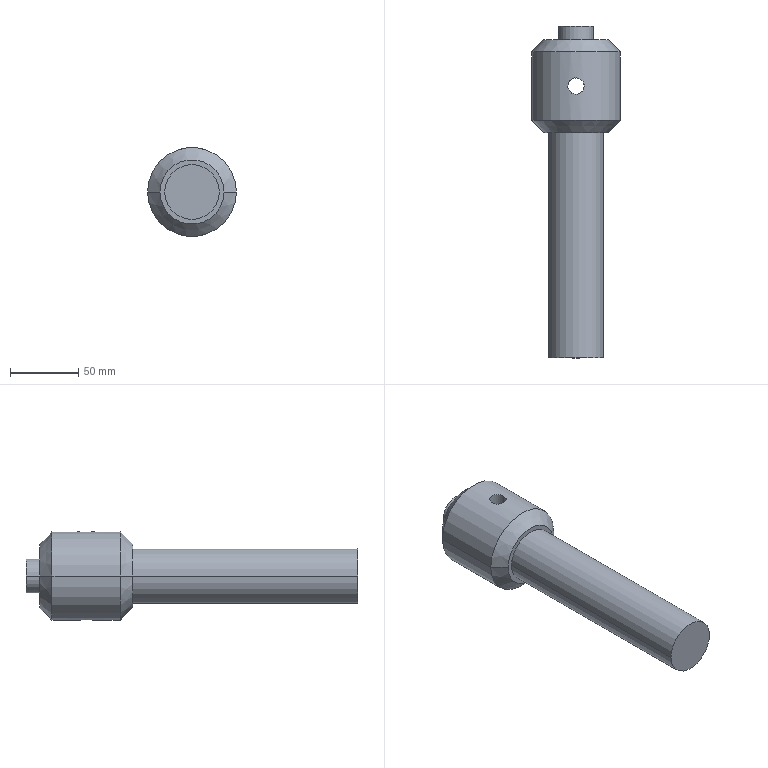Part | SolidWorks | features ICE 1, RevCut 1, Revolution 1 | 1 solid | 20 faces | box 65 x 243 x 65 mm | volume 412398 mm3 | cylinder 10 | cone 6 | plane 4 | commonest cylinder face diameters 12 x4 25 x2 40 x2 65 x2
STEP:
#1=CARTESIAN_POINT('',(-6.,7.625,-31.941));
#2=VERTEX_POINT('',#1);
#3=CARTESIAN_POINT('',(6.,7.625,-31.941));
#4=VERTEX_POINT('',#3);
#5=CARTESIAN_POINT('',(-6.,7.625,-31.941));
#6=CARTESIAN_POINT('',(-6.,7.233,-31.941));
#7=CARTESIAN_POINT('',(-5.962,6.843,-31.949));
#8=CARTESIAN_POINT('',(-5.808,6.066,-31.977));
#9=CARTESIAN_POINT('',(-5.693,5.689,-31.998));
#10=CARTESIAN_POINT('',(-5.468,5.147,-32.037));
#11=CARTESIAN_POINT('',(-5.384,4.97,-32.051));
#12=CARTESIAN_POINT('',(-5.199,4.624,-32.082));
#13=CARTESIAN_POINT('',(-5.097,4.453,-32.098));
#14=CARTESIAN_POINT('',(-4.769,3.963,-32.149));
#15=CARTESIAN_POINT('',(-4.522,3.662,-32.185));
#16=CARTESIAN_POINT('',(-3.969,3.108,-32.258));
#17=CARTESIAN_POINT('',(-3.661,2.855,-32.295));
#18=CARTESIAN_POINT('',(-3.011,2.421,-32.362));
#19=CARTESIAN_POINT('',(-2.667,2.236,-32.392));
#20=CARTESIAN_POINT('',(-2.121,2.009,-32.431));
#21=CARTESIAN_POINT('',(-1.934,1.942,-32.443));
#22=CARTESIAN_POINT('',(-1.558,1.827,-32.463));
#23=CARTESIAN_POINT('',(-1.368,1.78,-32.472));
#24=CARTESIAN_POINT('',(-0.7922,1.665,-32.493));
#25=CARTESIAN_POINT('',(-0.3995,1.625,-32.5));
#26=CARTESIAN_POINT('',(0.393,1.625,-32.5));
#27=CARTESIAN_POINT('',(0.7831,1.663,-32.493));
#28=CARTESIAN_POINT('',(1.552,1.816,-32.465));
#29=CARTESIAN_POINT('',(1.934,1.932,-32.444));
#30=CARTESIAN_POINT('',(2.659,2.232,-32.393));
#31=CARTESIAN_POINT('',(3.004,2.416,-32.363));
#32=CARTESIAN_POINT('',(3.493,2.743,-32.312));
#33=CARTESIAN_POINT('',(3.653,2.861,-32.294));
#34=CARTESIAN_POINT('',(3.957,3.11,-32.259));
#35=CARTESIAN_POINT('',(4.102,3.242,-32.24));
#36=CARTESIAN_POINT('',(4.516,3.655,-32.186));
#37=CARTESIAN_POINT('',(4.765,3.957,-32.15));
#38=CARTESIAN_POINT('',(5.205,4.614,-32.081));
#39=CARTESIAN_POINT('',(5.39,4.959,-32.05));
#40=CARTESIAN_POINT('',(5.615,5.501,-32.011));
#41=CARTESIAN_POINT('',(5.681,5.685,-32.));
#42=CARTESIAN_POINT('',(5.796,6.061,-31.979));
#43=CARTESIAN_POINT('',(5.845,6.255,-31.97));
#44=CARTESIAN_POINT('',(5.961,6.836,-31.949));
#45=CARTESIAN_POINT('',(6.,7.228,-31.941));
#46=CARTESIAN_POINT('',(6.,7.625,-31.941));
#47=B_SPLINE_CURVE_WITH_KNOTS('',3,(#5,#6,#7,#8,#9,#10,#11,#12,#13,#14,#15,#16,#17,#18,#19,#20,#21,#22,#23,#24,#25,#26,#27,#28,#29,#30,#31,#32,#33,#34,#35,#36,#37,#38,#39,#40,#41,#42,#43,#44,#45,#46),.UNSPECIFIED.,.F.,.F.,(4,2,2,2,2,2,2,2,2,2,2,2,2,2,2,2,2,2,2,2,4),(0.0188,0.01997,0.02115,0.02174,0.02232,0.0235,0.02467,0.02585,0.02643,0.02702,0.0282,0.02937,0.03055,0.03172,0.03231,0.03289,0.03407,0.03524,0.03583,0.03642,0.03759),.UNSPECIFIED.);
#48=EDGE_CURVE('',#2,#4,#47,.T.);
#49=ORIENTED_EDGE('',*,*,#48,.F.);
#50=CARTESIAN_POINT('',(-6.,7.625,31.941));
#51=VERTEX_POINT('',#50);
#52=CARTESIAN_POINT('',(-6.,7.625,-80.));
#53=DIRECTION('',(0.,0.,1.));
#54=VECTOR('',#53,1000.);
#55=LINE('',#52,#54);
#56=EDGE_CURVE('',#2,#51,#55,.T.);
#57=ORIENTED_EDGE('',*,*,#56,.T.);
#58=CARTESIAN_POINT('',(6.,7.625,31.941));
#59=VERTEX_POINT('',#58);
#60=CARTESIAN_POINT('',(6.,7.625,31.941));
#61=CARTESIAN_POINT('',(6.,7.228,31.941));
#62=CARTESIAN_POINT('',(5.961,6.837,31.949));
#63=CARTESIAN_POINT('',(5.846,6.261,31.97));
#64=CARTESIAN_POINT('',(5.799,6.071,31.979));
#65=CARTESIAN_POINT('',(5.684,5.693,31.999));
#66=CARTESIAN_POINT('',(5.617,5.506,32.011));
#67=CARTESIAN_POINT('',(5.391,4.961,32.05));
#68=CARTESIAN_POINT('',(5.206,4.617,32.081));
#69=CARTESIAN_POINT('',(4.771,3.965,32.149));
#70=CARTESIAN_POINT('',(4.518,3.658,32.186));
#71=CARTESIAN_POINT('',(3.966,3.105,32.258));
#72=CARTESIAN_POINT('',(3.664,2.857,32.294));
#73=CARTESIAN_POINT('',(3.008,2.419,32.362));
#74=CARTESIAN_POINT('',(2.66,2.233,32.393));
#75=CARTESIAN_POINT('',(2.119,2.008,32.431));
#76=CARTESIAN_POINT('',(1.935,1.942,32.443));
#77=CARTESIAN_POINT('',(1.559,1.828,32.463));
#78=CARTESIAN_POINT('',(1.366,1.779,32.472));
#79=CARTESIAN_POINT('',(0.7845,1.663,32.493));
#80=CARTESIAN_POINT('',(0.3946,1.625,32.5));
#81=CARTESIAN_POINT('',(-0.39,1.625,32.5));
#82=CARTESIAN_POINT('',(-0.7886,1.664,32.493));
#83=CARTESIAN_POINT('',(-1.559,1.818,32.465));
#84=CARTESIAN_POINT('',(-1.933,1.931,32.445));
#85=CARTESIAN_POINT('',(-2.479,2.157,32.406));
#86=CARTESIAN_POINT('',(-2.659,2.243,32.392));
#87=CARTESIAN_POINT('',(-3.005,2.428,32.361));
#88=CARTESIAN_POINT('',(-3.173,2.529,32.345));
#89=CARTESIAN_POINT('',(-3.66,2.854,32.295));
#90=CARTESIAN_POINT('',(-3.964,3.104,32.259));
#91=CARTESIAN_POINT('',(-4.522,3.662,32.185));
#92=CARTESIAN_POINT('',(-4.77,3.964,32.149));
#93=CARTESIAN_POINT('',(-5.095,4.451,32.098));
#94=CARTESIAN_POINT('',(-5.196,4.619,32.082));
#95=CARTESIAN_POINT('',(-5.382,4.966,32.051));
#96=CARTESIAN_POINT('',(-5.467,5.146,32.037));
#97=CARTESIAN_POINT('',(-5.693,5.69,31.998));
#98=CARTESIAN_POINT('',(-5.807,6.064,31.977));
#99=CARTESIAN_POINT('',(-5.961,6.835,31.949));
#100=CARTESIAN_POINT('',(-6.,7.233,31.941));
#101=CARTESIAN_POINT('',(-6.,7.625,31.941));
#102=B_SPLINE_CURVE_WITH_KNOTS('',3,(#60,#61,#62,#63,#64,#65,#66,#67,#68,#69,#70,#71,#72,#73,#74,#75,#76,#77,#78,#79,#80,#81,#82,#83,#84,#85,#86,#87,#88,#89,#90,#91,#92,#93,#94,#95,#96,#97,#98,#99,#100,#101),.UNSPECIFIED.,.F.,.F.,(4,2,2,2,2,2,2,2,2,2,2,2,2,2,2,2,2,2,2,2,4),(0.,0.001175,0.001762,0.00235,0.003525,0.0047,0.005875,0.00705,0.007637,0.008225,0.0094,0.01057,0.01175,0.01234,0.01292,0.0141,0.01527,0.01586,0.01645,0.01762,0.0188),.UNSPECIFIED.);
#103=EDGE_CURVE('',#59,#51,#102,.T.);
#104=ORIENTED_EDGE('',*,*,#103,.F.);
#105=CARTESIAN_POINT('',(6.,7.625,-80.));
#106=DIRECTION('',(0.,0.,1.));
#107=VECTOR('',#106,1000.);
#108=LINE('',#105,#107);
#109=EDGE_CURVE('',#4,#59,#108,.T.);
#110=ORIENTED_EDGE('',*,*,#109,.F.);
#111=EDGE_LOOP('',(#49,#57,#104,#110));
#112=FACE_OUTER_BOUND('',#111,.T.);
#113=CARTESIAN_POINT('',(0.,7.625,-80.));
#114=DIRECTION('',(0.,0.,1.));
#115=DIRECTION('',(1.,0.,0.));
#116=AXIS2_PLACEMENT_3D('',#113,#114,#115);
#117=CYLINDRICAL_SURFACE('',#116,6.);
#118=ADVANCED_FACE('',(#112),#117,.F.);
#119=CARTESIAN_POINT('',(0.,21.625,0.));
#120=VERTEX_POINT('',#119);
#121=CARTESIAN_POINT('',(-6.,24.625,0.));
#122=VERTEX_POINT('',#121);
#123=CARTESIAN_POINT('',(0.,21.625,0.));
#124=DIRECTION('',(-0.8944,0.4472,0.));
#125=VECTOR('',#124,1000.);
#126=LINE('',#123,#125);
#127=EDGE_CURVE('',#120,#122,#126,.T.);
#128=ORIENTED_EDGE('',*,*,#127,.F.);
#129=CARTESIAN_POINT('',(6.,24.625,0.));
#130=VERTEX_POINT('',#129);
#131=CARTESIAN_POINT('',(0.,21.625,0.));
#132=DIRECTION('',(0.8944,0.4472,0.));
#133=VECTOR('',#132,1000.);
#134=LINE('',#131,#133);
#135=EDGE_CURVE('',#120,#130,#134,.T.);
#136=ORIENTED_EDGE('',*,*,#135,.T.);
#137=CARTESIAN_POINT('',(0.,24.625,0.));
#138=DIRECTION('',(0.,1.,0.));
#139=DIRECTION('',(-1.,0.,0.));
#140=AXIS2_PLACEMENT_3D('',#137,#138,#139);
#141=CIRCLE('',#140,6.);
#142=EDGE_CURVE('',#130,#122,#141,.T.);
#143=ORIENTED_EDGE('',*,*,#142,.T.);
#144=EDGE_LOOP('',(#128,#136,#143));
#145=FACE_OUTER_BOUND('',#144,.T.);
#146=CARTESIAN_POINT('',(0.,1021.625,0.));
#147=DIRECTION('',(0.,1.,0.));
#148=DIRECTION('',(-1.,0.,0.));
#149=AXIS2_PLACEMENT_3D('',#146,#147,#148);
#150=CONICAL_SURFACE('',#149,2000.,1.107);
#151=ADVANCED_FACE('',(#145),#150,.F.);
#152=ORIENTED_EDGE('',*,*,#142,.F.);
#153=CARTESIAN_POINT('',(6.,51.625,0.));
#154=VERTEX_POINT('',#153);
#155=CARTESIAN_POINT('',(6.,51.625,0.));
#156=DIRECTION('',(0.,1.,0.));
#157=VECTOR('',#156,1000.);
#158=LINE('',#155,#157);
#159=EDGE_CURVE('',#130,#154,#158,.T.);
#160=ORIENTED_EDGE('',*,*,#159,.T.);
#161=CARTESIAN_POINT('',(-6.,51.625,0.));
#162=VERTEX_POINT('',#161);
#163=CARTESIAN_POINT('',(0.,51.625,0.));
#164=DIRECTION('',(0.,1.,0.));
#165=DIRECTION('',(-1.,0.,0.));
#166=AXIS2_PLACEMENT_3D('',#163,#164,#165);
#167=CIRCLE('',#166,6.);
#168=EDGE_CURVE('',#154,#162,#167,.T.);
#169=ORIENTED_EDGE('',*,*,#168,.T.);
#170=CARTESIAN_POINT('',(-6.,51.625,0.));
#171=DIRECTION('',(0.,1.,0.));
#172=VECTOR('',#171,1000.);
#173=LINE('',#170,#172);
#174=EDGE_CURVE('',#122,#162,#173,.T.);
#175=ORIENTED_EDGE('',*,*,#174,.F.);
#176=EDGE_LOOP('',(#152,#160,#169,#175));
#177=FACE_OUTER_BOUND('',#176,.T.);
#178=CARTESIAN_POINT('',(0.,51.625,0.));
#179=DIRECTION('',(0.,1.,0.));
#180=DIRECTION('',(-1.,0.,0.));
#181=AXIS2_PLACEMENT_3D('',#178,#179,#180);
#182=CYLINDRICAL_SURFACE('',#181,6.);
#183=ADVANCED_FACE('',(#177),#182,.F.);
#184=CARTESIAN_POINT('',(-12.5,41.625,0.));
#185=VERTEX_POINT('',#184);
#186=CARTESIAN_POINT('',(12.5,41.625,0.));
#187=VERTEX_POINT('',#186);
#188=CARTESIAN_POINT('',(0.,41.625,0.));
#189=DIRECTION('',(0.,1.,0.));
#190=DIRECTION('',(-1.,0.,0.));
#191=AXIS2_PLACEMENT_3D('',#188,#189,#190);
#192=CIRCLE('',#191,12.5);
#193=EDGE_CURVE('',#185,#187,#192,.T.);
#194=ORIENTED_EDGE('',*,*,#193,.T.);
#195=CARTESIAN_POINT('',(12.5,51.625,0.));
#196=VERTEX_POINT('',#195);
#197=CARTESIAN_POINT('',(12.5,-26.375,0.));
#198=DIRECTION('',(0.,1.,0.));
#199=VECTOR('',#198,1000.);
#200=LINE('',#197,#199);
#201=EDGE_CURVE('',#187,#196,#200,.T.);
#202=ORIENTED_EDGE('',*,*,#201,.T.);
#203=CARTESIAN_POINT('',(-12.5,51.625,0.));
#204=VERTEX_POINT('',#203);
#205=CARTESIAN_POINT('',(0.,51.625,0.));
#206=DIRECTION('',(0.,1.,0.));
#207=DIRECTION('',(-1.,0.,0.));
#208=AXIS2_PLACEMENT_3D('',#205,#206,#207);
#209=CIRCLE('',#208,12.5);
#210=EDGE_CURVE('',#204,#196,#209,.T.);
#211=ORIENTED_EDGE('',*,*,#210,.F.);
#212=CARTESIAN_POINT('',(-12.5,-26.375,0.));
#213=DIRECTION('',(0.,1.,0.));
#214=VECTOR('',#213,1000.);
#215=LINE('',#212,#214);
#216=EDGE_CURVE('',#185,#204,#215,.T.);
#217=ORIENTED_EDGE('',*,*,#216,.F.);
#218=EDGE_LOOP('',(#194,#202,#211,#217));
#219=FACE_OUTER_BOUND('',#218,.T.);
#220=CARTESIAN_POINT('',(0.,-26.375,0.));
#221=DIRECTION('',(0.,1.,0.));
#222=DIRECTION('',(-1.,0.,0.));
#223=AXIS2_PLACEMENT_3D('',#220,#221,#222);
#224=CYLINDRICAL_SURFACE('',#223,12.5);
#225=ADVANCED_FACE('',(#219),#224,.T.);
#226=CARTESIAN_POINT('',(-23.5,41.625,0.));
#227=VERTEX_POINT('',#226);
#228=CARTESIAN_POINT('',(23.5,41.625,0.));
#229=VERTEX_POINT('',#228);
#230=CARTESIAN_POINT('',(0.,41.625,0.));
#231=DIRECTION('',(0.,1.,0.));
#232=DIRECTION('',(-1.,0.,0.));
#233=AXIS2_PLACEMENT_3D('',#230,#231,#232);
#234=CIRCLE('',#233,23.5);
#235=EDGE_CURVE('',#227,#229,#234,.T.);
#236=ORIENTED_EDGE('',*,*,#235,.F.);
#237=CARTESIAN_POINT('',(-32.5,32.625,0.));
#238=VERTEX_POINT('',#237);
#239=CARTESIAN_POINT('',(-23.5,41.625,0.));
#240=DIRECTION('',(-0.7071,-0.7071,0.));
#241=VECTOR('',#240,1000.);
#242=LINE('',#239,#241);
#243=EDGE_CURVE('',#227,#238,#242,.T.);
#244=ORIENTED_EDGE('',*,*,#243,.T.);
#245=CARTESIAN_POINT('',(32.5,32.625,0.));
#246=VERTEX_POINT('',#245);
#247=CARTESIAN_POINT('',(0.,32.625,0.));
#248=DIRECTION('',(0.,1.,0.));
#249=DIRECTION('',(-1.,0.,0.));
#250=AXIS2_PLACEMENT_3D('',#247,#248,#249);
#251=CIRCLE('',#250,32.5);
#252=EDGE_CURVE('',#238,#246,#251,.T.);
#253=ORIENTED_EDGE('',*,*,#252,.T.);
#254=CARTESIAN_POINT('',(23.5,41.625,0.));
#255=DIRECTION('',(0.7071,-0.7071,0.));
#256=VECTOR('',#255,1000.);
#257=LINE('',#254,#256);
#258=EDGE_CURVE('',#229,#246,#257,.T.);
#259=ORIENTED_EDGE('',*,*,#258,.F.);
#260=EDGE_LOOP('',(#236,#244,#253,#259));
#261=FACE_OUTER_BOUND('',#260,.T.);
#262=CARTESIAN_POINT('',(0.,41.625,0.));
#263=DIRECTION('',(0.,-1.,0.));
#264=DIRECTION('',(1.,0.,0.));
#265=AXIS2_PLACEMENT_3D('',#262,#263,#264);
#266=CONICAL_SURFACE('',#265,23.5,0.7854);
#267=ADVANCED_FACE('',(#261),#266,.T.);
#268=ORIENTED_EDGE('',*,*,#103,.T.);
#269=CARTESIAN_POINT('',(-6.,7.625,31.941));
#270=CARTESIAN_POINT('',(-6.,8.017,31.941));
#271=CARTESIAN_POINT('',(-5.962,8.407,31.949));
#272=CARTESIAN_POINT('',(-5.808,9.184,31.977));
#273=CARTESIAN_POINT('',(-5.693,9.561,31.998));
#274=CARTESIAN_POINT('',(-5.468,10.103,32.037));
#275=CARTESIAN_POINT('',(-5.384,10.28,32.051));
#276=CARTESIAN_POINT('',(-5.199,10.626,32.082));
#277=CARTESIAN_POINT('',(-5.097,10.797,32.098));
#278=CARTESIAN_POINT('',(-4.769,11.287,32.149));
#279=CARTESIAN_POINT('',(-4.522,11.588,32.185));
#280=CARTESIAN_POINT('',(-3.969,12.142,32.258));
#281=CARTESIAN_POINT('',(-3.661,12.395,32.295));
#282=CARTESIAN_POINT('',(-3.011,12.829,32.362));
#283=CARTESIAN_POINT('',(-2.667,13.014,32.392));
#284=CARTESIAN_POINT('',(-2.121,13.241,32.431));
#285=CARTESIAN_POINT('',(-1.934,13.308,32.443));
#286=CARTESIAN_POINT('',(-1.558,13.423,32.463));
#287=CARTESIAN_POINT('',(-1.368,13.47,32.472));
#288=CARTESIAN_POINT('',(-0.7922,13.585,32.493));
#289=CARTESIAN_POINT('',(-0.3995,13.625,32.5));
#290=CARTESIAN_POINT('',(0.393,13.625,32.5));
#291=CARTESIAN_POINT('',(0.7831,13.587,32.493));
#292=CARTESIAN_POINT('',(1.552,13.434,32.465));
#293=CARTESIAN_POINT('',(1.934,13.318,32.444));
#294=CARTESIAN_POINT('',(2.659,13.018,32.393));
#295=CARTESIAN_POINT('',(3.004,12.834,32.363));
#296=CARTESIAN_POINT('',(3.493,12.507,32.312));
#297=CARTESIAN_POINT('',(3.653,12.389,32.294));
#298=CARTESIAN_POINT('',(3.957,12.14,32.259));
#299=CARTESIAN_POINT('',(4.102,12.008,32.24));
#300=CARTESIAN_POINT('',(4.516,11.595,32.186));
#301=CARTESIAN_POINT('',(4.765,11.293,32.15));
#302=CARTESIAN_POINT('',(5.205,10.636,32.081));
#303=CARTESIAN_POINT('',(5.39,10.291,32.05));
#304=CARTESIAN_POINT('',(5.615,9.749,32.011));
#305=CARTESIAN_POINT('',(5.681,9.565,32.));
#306=CARTESIAN_POINT('',(5.796,9.189,31.979));
#307=CARTESIAN_POINT('',(5.845,8.995,31.97));
#308=CARTESIAN_POINT('',(5.961,8.414,31.949));
#309=CARTESIAN_POINT('',(6.,8.022,31.941));
#310=CARTESIAN_POINT('',(6.,7.625,31.941));
#311=B_SPLINE_CURVE_WITH_KNOTS('',3,(#269,#270,#271,#272,#273,#274,#275,#276,#277,#278,#279,#280,#281,#282,#283,#284,#285,#286,#287,#288,#289,#290,#291,#292,#293,#294,#295,#296,#297,#298,#299,#300,#301,#302,#303,#304,#305,#306,#307,#308,#309,#310),.UNSPECIFIED.,.F.,.F.,(4,2,2,2,2,2,2,2,2,2,2,2,2,2,2,2,2,2,2,2,4),(0.0188,0.01997,0.02115,0.02174,0.02232,0.0235,0.02467,0.02585,0.02643,0.02702,0.0282,0.02937,0.03055,0.03172,0.03231,0.03289,0.03407,0.03524,0.03583,0.03642,0.03759),.UNSPECIFIED.);
#312=EDGE_CURVE('',#51,#59,#311,.T.);
#313=ORIENTED_EDGE('',*,*,#312,.T.);
#314=EDGE_LOOP('',(#268,#313));
#315=FACE_BOUND('',#314,.T.);
#316=CARTESIAN_POINT('',(-32.5,-17.375,0.));
#317=VERTEX_POINT('',#316);
#318=CARTESIAN_POINT('',(32.5,-17.375,0.));
#319=VERTEX_POINT('',#318);
#320=CARTESIAN_POINT('',(0.,-17.375,0.));
#321=DIRECTION('',(0.,1.,0.));
#322=DIRECTION('',(-1.,0.,0.));
#323=AXIS2_PLACEMENT_3D('',#320,#321,#322);
#324=CIRCLE('',#323,32.5);
#325=EDGE_CURVE('',#317,#319,#324,.T.);
#326=ORIENTED_EDGE('',*,*,#325,.T.);
#327=CARTESIAN_POINT('',(32.5,-26.375,0.));
#328=DIRECTION('',(0.,1.,0.));
#329=VECTOR('',#328,1000.);
#330=LINE('',#327,#329);
#331=EDGE_CURVE('',#319,#246,#330,.T.);
#332=ORIENTED_EDGE('',*,*,#331,.T.);
#333=ORIENTED_EDGE('',*,*,#252,.F.);
#334=CARTESIAN_POINT('',(-32.5,-26.375,0.));
#335=DIRECTION('',(0.,1.,0.));
#336=VECTOR('',#335,1000.);
#337=LINE('',#334,#336);
#338=EDGE_CURVE('',#317,#238,#337,.T.);
#339=ORIENTED_EDGE('',*,*,#338,.F.);
#340=EDGE_LOOP('',(#326,#332,#333,#339));
#341=FACE_OUTER_BOUND('',#340,.T.);
#342=CARTESIAN_POINT('',(0.,-26.375,0.));
#343=DIRECTION('',(0.,1.,0.));
#344=DIRECTION('',(-1.,0.,0.));
#345=AXIS2_PLACEMENT_3D('',#342,#343,#344);
#346=CYLINDRICAL_SURFACE('',#345,32.5);
#347=ADVANCED_FACE('',(#315,#341),#346,.T.);
#348=CARTESIAN_POINT('',(-23.5,-26.375,0.));
#349=VERTEX_POINT('',#348);
#350=CARTESIAN_POINT('',(23.5,-26.375,0.));
#351=VERTEX_POINT('',#350);
#352=CARTESIAN_POINT('',(0.,-26.375,0.));
#353=DIRECTION('',(0.,1.,0.));
#354=DIRECTION('',(-1.,0.,0.));
#355=AXIS2_PLACEMENT_3D('',#352,#353,#354);
#356=CIRCLE('',#355,23.5);
#357=EDGE_CURVE('',#349,#351,#356,.T.);
#358=ORIENTED_EDGE('',*,*,#357,.T.);
#359=CARTESIAN_POINT('',(23.5,-26.375,0.));
#360=DIRECTION('',(0.7071,0.7071,0.));
#361=VECTOR('',#360,1000.);
#362=LINE('',#359,#361);
#363=EDGE_CURVE('',#351,#319,#362,.T.);
#364=ORIENTED_EDGE('',*,*,#363,.T.);
#365=ORIENTED_EDGE('',*,*,#325,.F.);
#366=CARTESIAN_POINT('',(-23.5,-26.375,0.));
#367=DIRECTION('',(-0.7071,0.7071,0.));
#368=VECTOR('',#367,1000.);
#369=LINE('',#366,#368);
#370=EDGE_CURVE('',#349,#317,#369,.T.);
#371=ORIENTED_EDGE('',*,*,#370,.F.);
#372=EDGE_LOOP('',(#358,#364,#365,#371));
#373=FACE_OUTER_BOUND('',#372,.T.);
#374=CARTESIAN_POINT('',(0.,-26.375,0.));
#375=DIRECTION('',(0.,1.,0.));
#376=DIRECTION('',(-1.,0.,0.));
#377=AXIS2_PLACEMENT_3D('',#374,#375,#376);
#378=CONICAL_SURFACE('',#377,23.5,0.7854);
#379=ADVANCED_FACE('',(#373),#378,.T.);
#380=CARTESIAN_POINT('',(-20.,-191.375,0.));
#381=VERTEX_POINT('',#380);
#382=CARTESIAN_POINT('',(20.,-191.375,0.));
#383=VERTEX_POINT('',#382);
#384=CARTESIAN_POINT('',(0.,-191.375,0.));
#385=DIRECTION('',(0.,1.,0.));
#386=DIRECTION('',(-1.,0.,0.));
#387=AXIS2_PLACEMENT_3D('',#384,#385,#386);
#388=CIRCLE('',#387,20.);
#389=EDGE_CURVE('',#381,#383,#388,.T.);
#390=ORIENTED_EDGE('',*,*,#389,.T.);
#391=CARTESIAN_POINT('',(20.,-26.375,0.));
#392=VERTEX_POINT('',#391);
#393=CARTESIAN_POINT('',(20.,-26.375,0.));
#394=DIRECTION('',(0.,1.,0.));
#395=VECTOR('',#394,1000.);
#396=LINE('',#393,#395);
#397=EDGE_CURVE('',#383,#392,#396,.T.);
#398=ORIENTED_EDGE('',*,*,#397,.T.);
#399=CARTESIAN_POINT('',(-20.,-26.375,0.));
#400=VERTEX_POINT('',#399);
#401=CARTESIAN_POINT('',(0.,-26.375,0.));
#402=DIRECTION('',(0.,1.,0.));
#403=DIRECTION('',(-1.,0.,0.));
#404=AXIS2_PLACEMENT_3D('',#401,#402,#403);
#405=CIRCLE('',#404,20.);
#406=EDGE_CURVE('',#400,#392,#405,.T.);
#407=ORIENTED_EDGE('',*,*,#406,.F.);
#408=CARTESIAN_POINT('',(-20.,-26.375,0.));
#409=DIRECTION('',(0.,1.,0.));
#410=VECTOR('',#409,1000.);
#411=LINE('',#408,#410);
#412=EDGE_CURVE('',#381,#400,#411,.T.);
#413=ORIENTED_EDGE('',*,*,#412,.F.);
#414=EDGE_LOOP('',(#390,#398,#407,#413));
#415=FACE_OUTER_BOUND('',#414,.T.);
#416=CARTESIAN_POINT('',(0.,-26.375,0.));
#417=DIRECTION('',(0.,1.,0.));
#418=DIRECTION('',(-1.,0.,0.));
#419=AXIS2_PLACEMENT_3D('',#416,#417,#418);
#420=CYLINDRICAL_SURFACE('',#419,20.);
#421=ADVANCED_FACE('',(#415),#420,.T.);
#422=ORIENTED_EDGE('',*,*,#210,.T.);
#423=CARTESIAN_POINT('',(0.,51.625,0.));
#424=DIRECTION('',(0.,1.,0.));
#425=DIRECTION('',(-1.,0.,0.));
#426=AXIS2_PLACEMENT_3D('',#423,#424,#425);
#427=CIRCLE('',#426,12.5);
#428=EDGE_CURVE('',#196,#204,#427,.T.);
#429=ORIENTED_EDGE('',*,*,#428,.T.);
#430=EDGE_LOOP('',(#422,#429));
#431=FACE_OUTER_BOUND('',#430,.T.);
#432=CARTESIAN_POINT('',(0.,51.625,0.));
#433=DIRECTION('',(0.,1.,0.));
#434=DIRECTION('',(-1.,0.,0.));
#435=AXIS2_PLACEMENT_3D('',#432,#433,#434);
#436=CIRCLE('',#435,6.);
#437=EDGE_CURVE('',#162,#154,#436,.T.);
#438=ORIENTED_EDGE('',*,*,#437,.F.);
#439=ORIENTED_EDGE('',*,*,#168,.F.);
#440=EDGE_LOOP('',(#438,#439));
#441=FACE_BOUND('',#440,.T.);
#442=CARTESIAN_POINT('',(0.,51.625,0.));
#443=DIRECTION('',(0.,1.,0.));
#444=DIRECTION('',(-1.,0.,0.));
#445=AXIS2_PLACEMENT_3D('',#442,#443,#444);
#446=PLANE('',#445);
#447=ADVANCED_FACE('',(#431,#441),#446,.T.);
#448=ORIENTED_EDGE('',*,*,#389,.F.);
#449=CARTESIAN_POINT('',(0.,-191.375,0.));
#450=DIRECTION('',(0.,1.,0.));
#451=DIRECTION('',(-1.,0.,0.));
#452=AXIS2_PLACEMENT_3D('',#449,#450,#451);
#453=CIRCLE('',#452,20.);
#454=EDGE_CURVE('',#383,#381,#453,.T.);
#455=ORIENTED_EDGE('',*,*,#454,.F.);
#456=EDGE_LOOP('',(#448,#455));
#457=FACE_OUTER_BOUND('',#456,.T.);
#458=CARTESIAN_POINT('',(0.,-191.375,0.));
#459=DIRECTION('',(0.,1.,0.));
#460=DIRECTION('',(-1.,0.,0.));
#461=AXIS2_PLACEMENT_3D('',#458,#459,#460);
#462=PLANE('',#461);
#463=ADVANCED_FACE('',(#457),#462,.F.);
#464=ORIENTED_EDGE('',*,*,#397,.F.);
#465=ORIENTED_EDGE('',*,*,#454,.T.);
#466=ORIENTED_EDGE('',*,*,#412,.T.);
#467=CARTESIAN_POINT('',(0.,-26.375,0.));
#468=DIRECTION('',(0.,1.,0.));
#469=DIRECTION('',(-1.,0.,0.));
#470=AXIS2_PLACEMENT_3D('',#467,#468,#469);
#471=CIRCLE('',#470,20.);
#472=EDGE_CURVE('',#392,#400,#471,.T.);
#473=ORIENTED_EDGE('',*,*,#472,.F.);
#474=EDGE_LOOP('',(#464,#465,#466,#473));
#475=FACE_OUTER_BOUND('',#474,.T.);
#476=CARTESIAN_POINT('',(0.,-26.375,0.));
#477=DIRECTION('',(0.,1.,0.));
#478=DIRECTION('',(-1.,0.,0.));
#479=AXIS2_PLACEMENT_3D('',#476,#477,#478);
#480=CYLINDRICAL_SURFACE('',#479,20.);
#481=ADVANCED_FACE('',(#475),#480,.T.);
#482=ORIENTED_EDGE('',*,*,#357,.F.);
#483=CARTESIAN_POINT('',(0.,-26.375,0.));
#484=DIRECTION('',(0.,1.,0.));
#485=DIRECTION('',(-1.,0.,0.));
#486=AXIS2_PLACEMENT_3D('',#483,#484,#485);
#487=CIRCLE('',#486,23.5);
#488=EDGE_CURVE('',#351,#349,#487,.T.);
#489=ORIENTED_EDGE('',*,*,#488,.F.);
#490=EDGE_LOOP('',(#482,#489));
#491=FACE_OUTER_BOUND('',#490,.T.);
#492=ORIENTED_EDGE('',*,*,#406,.T.);
#493=ORIENTED_EDGE('',*,*,#472,.T.);
#494=EDGE_LOOP('',(#492,#493));
#495=FACE_BOUND('',#494,.T.);
#496=CARTESIAN_POINT('',(0.,-26.375,0.));
#497=DIRECTION('',(0.,1.,0.));
#498=DIRECTION('',(-1.,0.,0.));
#499=AXIS2_PLACEMENT_3D('',#496,#497,#498);
#500=PLANE('',#499);
#501=ADVANCED_FACE('',(#491,#495),#500,.F.);
#502=ORIENTED_EDGE('',*,*,#363,.F.);
#503=ORIENTED_EDGE('',*,*,#488,.T.);
#504=ORIENTED_EDGE('',*,*,#370,.T.);
#505=CARTESIAN_POINT('',(0.,-17.375,0.));
#506=DIRECTION('',(0.,1.,0.));
#507=DIRECTION('',(-1.,0.,0.));
#508=AXIS2_PLACEMENT_3D('',#505,#506,#507);
#509=CIRCLE('',#508,32.5);
#510=EDGE_CURVE('',#319,#317,#509,.T.);
#511=ORIENTED_EDGE('',*,*,#510,.F.);
#512=EDGE_LOOP('',(#502,#503,#504,#511));
#513=FACE_OUTER_BOUND('',#512,.T.);
#514=CARTESIAN_POINT('',(0.,-26.375,0.));
#515=DIRECTION('',(0.,1.,0.));
#516=DIRECTION('',(-1.,0.,0.));
#517=AXIS2_PLACEMENT_3D('',#514,#515,#516);
#518=CONICAL_SURFACE('',#517,23.5,0.7854);
#519=ADVANCED_FACE('',(#513),#518,.T.);
#520=ORIENTED_EDGE('',*,*,#331,.F.);
#521=ORIENTED_EDGE('',*,*,#510,.T.);
#522=ORIENTED_EDGE('',*,*,#338,.T.);
#523=CARTESIAN_POINT('',(0.,32.625,0.));
#524=DIRECTION('',(0.,1.,0.));
#525=DIRECTION('',(-1.,0.,0.));
#526=AXIS2_PLACEMENT_3D('',#523,#524,#525);
#527=CIRCLE('',#526,32.5);
#528=EDGE_CURVE('',#246,#238,#527,.T.);
#529=ORIENTED_EDGE('',*,*,#528,.F.);
#530=EDGE_LOOP('',(#520,#521,#522,#529));
#531=FACE_OUTER_BOUND('',#530,.T.);
#532=CARTESIAN_POINT('',(6.,7.625,-31.941));
#533=CARTESIAN_POINT('',(6.,8.022,-31.941));
#534=CARTESIAN_POINT('',(5.961,8.413,-31.949));
#535=CARTESIAN_POINT('',(5.846,8.989,-31.97));
#536=CARTESIAN_POINT('',(5.799,9.179,-31.979));
#537=CARTESIAN_POINT('',(5.684,9.557,-31.999));
#538=CARTESIAN_POINT('',(5.617,9.744,-32.011));
#539=CARTESIAN_POINT('',(5.391,10.289,-32.05));
#540=CARTESIAN_POINT('',(5.206,10.633,-32.081));
#541=CARTESIAN_POINT('',(4.771,11.285,-32.149));
#542=CARTESIAN_POINT('',(4.518,11.592,-32.186));
#543=CARTESIAN_POINT('',(3.966,12.145,-32.258));
#544=CARTESIAN_POINT('',(3.664,12.393,-32.294));
#545=CARTESIAN_POINT('',(3.008,12.831,-32.362));
#546=CARTESIAN_POINT('',(2.66,13.017,-32.393));
#547=CARTESIAN_POINT('',(2.119,13.242,-32.431));
#548=CARTESIAN_POINT('',(1.935,13.308,-32.443));
#549=CARTESIAN_POINT('',(1.559,13.422,-32.463));
#550=CARTESIAN_POINT('',(1.366,13.471,-32.472));
#551=CARTESIAN_POINT('',(0.7845,13.587,-32.493));
#552=CARTESIAN_POINT('',(0.3946,13.625,-32.5));
#553=CARTESIAN_POINT('',(-0.39,13.625,-32.5));
#554=CARTESIAN_POINT('',(-0.7886,13.586,-32.493));
#555=CARTESIAN_POINT('',(-1.559,13.432,-32.465));
#556=CARTESIAN_POINT('',(-1.933,13.319,-32.445));
#557=CARTESIAN_POINT('',(-2.479,13.093,-32.406));
#558=CARTESIAN_POINT('',(-2.659,13.007,-32.392));
#559=CARTESIAN_POINT('',(-3.005,12.822,-32.361));
#560=CARTESIAN_POINT('',(-3.173,12.721,-32.345));
#561=CARTESIAN_POINT('',(-3.66,12.396,-32.295));
#562=CARTESIAN_POINT('',(-3.964,12.146,-32.259));
#563=CARTESIAN_POINT('',(-4.522,11.588,-32.185));
#564=CARTESIAN_POINT('',(-4.77,11.286,-32.149));
#565=CARTESIAN_POINT('',(-5.095,10.799,-32.098));
#566=CARTESIAN_POINT('',(-5.196,10.631,-32.082));
#567=CARTESIAN_POINT('',(-5.382,10.284,-32.051));
#568=CARTESIAN_POINT('',(-5.467,10.104,-32.037));
#569=CARTESIAN_POINT('',(-5.693,9.56,-31.998));
#570=CARTESIAN_POINT('',(-5.807,9.186,-31.977));
#571=CARTESIAN_POINT('',(-5.961,8.415,-31.949));
#572=CARTESIAN_POINT('',(-6.,8.017,-31.941));
#573=CARTESIAN_POINT('',(-6.,7.625,-31.941));
#574=B_SPLINE_CURVE_WITH_KNOTS('',3,(#532,#533,#534,#535,#536,#537,#538,#539,#540,#541,#542,#543,#544,#545,#546,#547,#548,#549,#550,#551,#552,#553,#554,#555,#556,#557,#558,#559,#560,#561,#562,#563,#564,#565,#566,#567,#568,#569,#570,#571,#572,#573),.UNSPECIFIED.,.F.,.F.,(4,2,2,2,2,2,2,2,2,2,2,2,2,2,2,2,2,2,2,2,4),(0.,0.001175,0.001762,0.00235,0.003525,0.0047,0.005875,0.00705,0.007637,0.008225,0.0094,0.01057,0.01175,0.01234,0.01292,0.0141,0.01527,0.01586,0.01645,0.01762,0.0188),.UNSPECIFIED.);
#575=EDGE_CURVE('',#4,#2,#574,.T.);
#576=ORIENTED_EDGE('',*,*,#575,.T.);
#577=ORIENTED_EDGE('',*,*,#48,.T.);
#578=EDGE_LOOP('',(#576,#577));
#579=FACE_BOUND('',#578,.T.);
#580=CARTESIAN_POINT('',(0.,-26.375,0.));
#581=DIRECTION('',(0.,1.,0.));
#582=DIRECTION('',(-1.,0.,0.));
#583=AXIS2_PLACEMENT_3D('',#580,#581,#582);
#584=CYLINDRICAL_SURFACE('',#583,32.5);
#585=ADVANCED_FACE('',(#531,#579),#584,.T.);
#586=ORIENTED_EDGE('',*,*,#243,.F.);
#587=CARTESIAN_POINT('',(0.,41.625,0.));
#588=DIRECTION('',(0.,1.,0.));
#589=DIRECTION('',(-1.,0.,0.));
#590=AXIS2_PLACEMENT_3D('',#587,#588,#589);
#591=CIRCLE('',#590,23.5);
#592=EDGE_CURVE('',#229,#227,#591,.T.);
#593=ORIENTED_EDGE('',*,*,#592,.F.);
#594=ORIENTED_EDGE('',*,*,#258,.T.);
#595=ORIENTED_EDGE('',*,*,#528,.T.);
#596=EDGE_LOOP('',(#586,#593,#594,#595));
#597=FACE_OUTER_BOUND('',#596,.T.);
#598=CARTESIAN_POINT('',(0.,41.625,0.));
#599=DIRECTION('',(0.,-1.,0.));
#600=DIRECTION('',(1.,0.,0.));
#601=AXIS2_PLACEMENT_3D('',#598,#599,#600);
#602=CONICAL_SURFACE('',#601,23.5,0.7854);
#603=ADVANCED_FACE('',(#597),#602,.T.);
#604=ORIENTED_EDGE('',*,*,#592,.T.);
#605=ORIENTED_EDGE('',*,*,#235,.T.);
#606=EDGE_LOOP('',(#604,#605));
#607=FACE_OUTER_BOUND('',#606,.T.);
#608=ORIENTED_EDGE('',*,*,#193,.F.);
#609=CARTESIAN_POINT('',(0.,41.625,0.));
#610=DIRECTION('',(0.,1.,0.));
#611=DIRECTION('',(-1.,0.,0.));
#612=AXIS2_PLACEMENT_3D('',#609,#610,#611);
#613=CIRCLE('',#612,12.5);
#614=EDGE_CURVE('',#187,#185,#613,.T.);
#615=ORIENTED_EDGE('',*,*,#614,.F.);
#616=EDGE_LOOP('',(#608,#615));
#617=FACE_BOUND('',#616,.T.);
#618=CARTESIAN_POINT('',(0.,41.625,0.));
#619=DIRECTION('',(0.,1.,0.));
#620=DIRECTION('',(-1.,0.,0.));
#621=AXIS2_PLACEMENT_3D('',#618,#619,#620);
#622=PLANE('',#621);
#623=ADVANCED_FACE('',(#607,#617),#622,.T.);
#624=ORIENTED_EDGE('',*,*,#201,.F.);
#625=ORIENTED_EDGE('',*,*,#614,.T.);
#626=ORIENTED_EDGE('',*,*,#216,.T.);
#627=ORIENTED_EDGE('',*,*,#428,.F.);
#628=EDGE_LOOP('',(#624,#625,#626,#627));
#629=FACE_OUTER_BOUND('',#628,.T.);
#630=CARTESIAN_POINT('',(0.,-26.375,0.));
#631=DIRECTION('',(0.,1.,0.));
#632=DIRECTION('',(-1.,0.,0.));
#633=AXIS2_PLACEMENT_3D('',#630,#631,#632);
#634=CYLINDRICAL_SURFACE('',#633,12.5);
#635=ADVANCED_FACE('',(#629),#634,.T.);
#636=ORIENTED_EDGE('',*,*,#159,.F.);
#637=CARTESIAN_POINT('',(0.,24.625,0.));
#638=DIRECTION('',(0.,1.,0.));
#639=DIRECTION('',(-1.,0.,0.));
#640=AXIS2_PLACEMENT_3D('',#637,#638,#639);
#641=CIRCLE('',#640,6.);
#642=EDGE_CURVE('',#122,#130,#641,.T.);
#643=ORIENTED_EDGE('',*,*,#642,.F.);
#644=ORIENTED_EDGE('',*,*,#174,.T.);
#645=ORIENTED_EDGE('',*,*,#437,.T.);
#646=EDGE_LOOP('',(#636,#643,#644,#645));
#647=FACE_OUTER_BOUND('',#646,.T.);
#648=CARTESIAN_POINT('',(0.,51.625,0.));
#649=DIRECTION('',(0.,1.,0.));
#650=DIRECTION('',(-1.,0.,0.));
#651=AXIS2_PLACEMENT_3D('',#648,#649,#650);
#652=CYLINDRICAL_SURFACE('',#651,6.);
#653=ADVANCED_FACE('',(#647),#652,.F.);
#654=ORIENTED_EDGE('',*,*,#135,.F.);
#655=ORIENTED_EDGE('',*,*,#127,.T.);
#656=ORIENTED_EDGE('',*,*,#642,.T.);
#657=EDGE_LOOP('',(#654,#655,#656));
#658=FACE_OUTER_BOUND('',#657,.T.);
#659=CARTESIAN_POINT('',(0.,1021.625,0.));
#660=DIRECTION('',(0.,1.,0.));
#661=DIRECTION('',(-1.,0.,0.));
#662=AXIS2_PLACEMENT_3D('',#659,#660,#661);
#663=CONICAL_SURFACE('',#662,2000.,1.107);
#664=ADVANCED_FACE('',(#658),#663,.F.);
#665=ORIENTED_EDGE('',*,*,#56,.F.);
#666=ORIENTED_EDGE('',*,*,#575,.F.);
#667=ORIENTED_EDGE('',*,*,#109,.T.);
#668=ORIENTED_EDGE('',*,*,#312,.F.);
#669=EDGE_LOOP('',(#665,#666,#667,#668));
#670=FACE_OUTER_BOUND('',#669,.T.);
#671=CARTESIAN_POINT('',(0.,7.625,-80.));
#672=DIRECTION('',(0.,0.,1.));
#673=DIRECTION('',(1.,0.,0.));
#674=AXIS2_PLACEMENT_3D('',#671,#672,#673);
#675=CYLINDRICAL_SURFACE('',#674,6.);
#676=ADVANCED_FACE('',(#670),#675,.F.);
#677=CLOSED_SHELL('',(#118,#151,#183,#225,#267,#347,#379,#421,#447,#463,#481,#501,#519,#585,#603,#623,#635,#653,#664,#676));
#678=MANIFOLD_SOLID_BREP('',#677);
#679=CARTESIAN_POINT('',(0.,0.,0.));
#680=DIRECTION('',(0.,0.,1.));
#681=DIRECTION('',(1.,0.,0.));
#682=AXIS2_PLACEMENT_3D('',#679,#680,#681);
#683=(LENGTH_UNIT()NAMED_UNIT(*)SI_UNIT(.MILLI.,.METRE.));
#684=UNCERTAINTY_MEASURE_WITH_UNIT(LENGTH_MEASURE(0.00001),#683,'','');
#685=(NAMED_UNIT(*)PLANE_ANGLE_UNIT()SI_UNIT($,.RADIAN.));
#686=(NAMED_UNIT(*)SI_UNIT($,.STERADIAN.)SOLID_ANGLE_UNIT());
#687=(GEOMETRIC_REPRESENTATION_CONTEXT(3)GLOBAL_UNCERTAINTY_ASSIGNED_CONTEXT((#684))GLOBAL_UNIT_ASSIGNED_CONTEXT((#683,#685,#686))REPRESENTATION_CONTEXT('',''));
#688=ADVANCED_BREP_SHAPE_REPRESENTATION('',(#678,#682),#687);